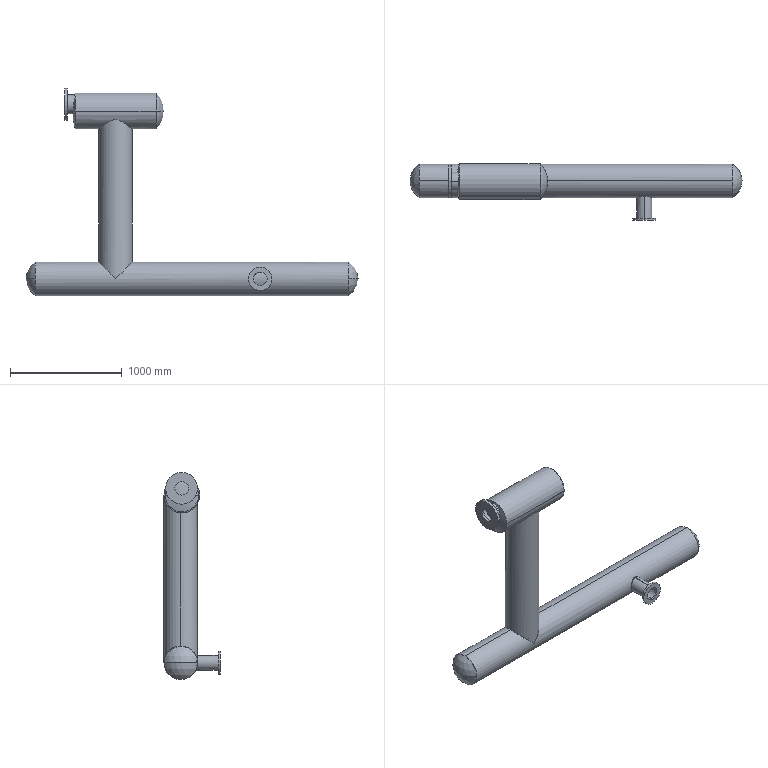Part | SolidWorks | features ICE 5, Revolution 2 | 1 solid | 84 faces | box 2968 x 502 x 1852 mm | volume 51909646 mm3 | cylinder 54 | torus 12 | plane 10 | sphere 8 | commonest cylinder face diameters 280 x13 300 x13 121 x6 133 x4 158 x4 170 x4